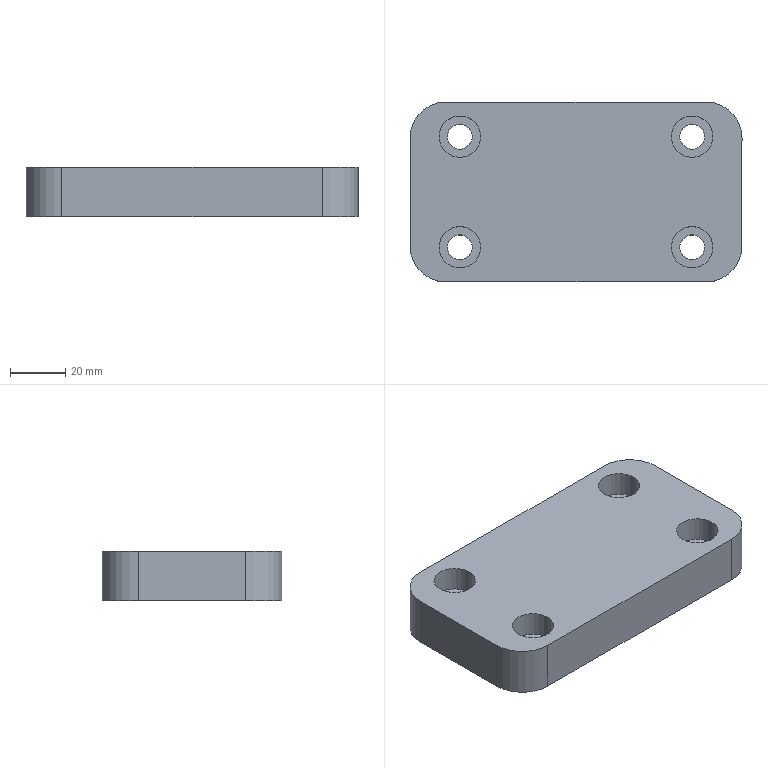Part | STEP file | solid 217 | 1 solid | 22 faces | box 120 x 65 x 18 mm | volume 129137 mm3 | cylinder 12 | plane 10 | commonest cylinder face diameters 9 x4 15 x4 26 x4